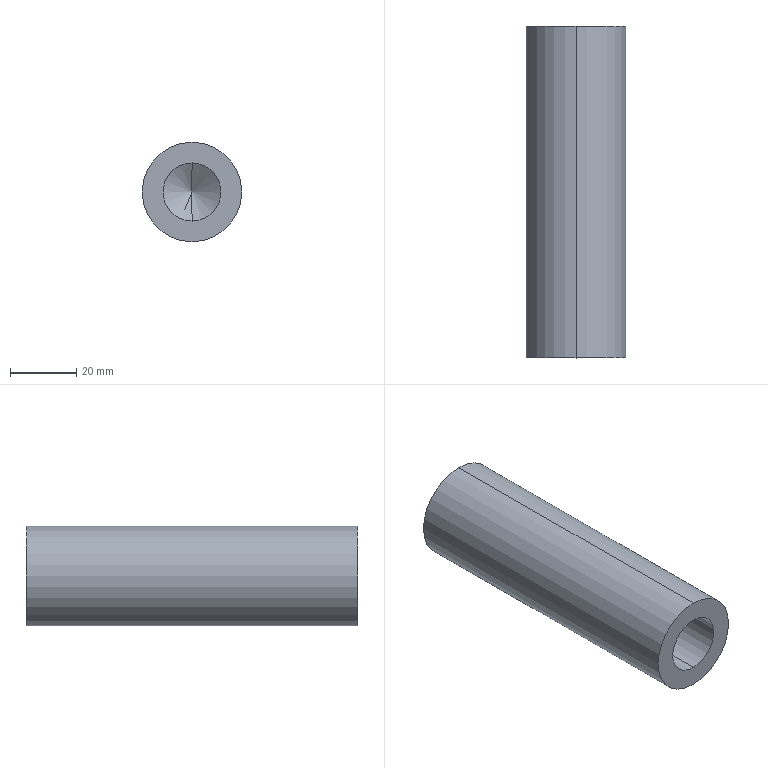Part | SolidWorks | features 3DProfileFeature 1, Extrusion 1, HoleWzd 1 | 1 solid | 8 faces | box 30 x 100 x 30 mm | volume 55231 mm3 | cylinder 4 | cone 2 | plane 2 | commonest cylinder face diameters 17.5 x2 30 x2
STEP:
#1=CARTESIAN_POINT('',(0.,12.5,8.75));
#2=VERTEX_POINT('',#1);
#3=CARTESIAN_POINT('',(0.,12.5,-8.75));
#4=VERTEX_POINT('',#3);
#5=CARTESIAN_POINT('',(0.,12.5,0.));
#6=DIRECTION('',(0.,-1.,0.));
#7=DIRECTION('',(0.,0.,-1.));
#8=AXIS2_PLACEMENT_3D('',#5,#6,#7);
#9=CIRCLE('',#8,8.75);
#10=EDGE_CURVE('',#2,#4,#9,.T.);
#11=ORIENTED_EDGE('',*,*,#10,.F.);
#12=CARTESIAN_POINT('',(0.,-50.,8.75));
#13=VERTEX_POINT('',#12);
#14=CARTESIAN_POINT('',(0.,-50.,8.75));
#15=DIRECTION('',(0.,-1.,0.));
#16=VECTOR('',#15,1000.);
#17=LINE('',#14,#16);
#18=EDGE_CURVE('',#2,#13,#17,.T.);
#19=ORIENTED_EDGE('',*,*,#18,.T.);
#20=CARTESIAN_POINT('',(0.,-50.,-8.75));
#21=VERTEX_POINT('',#20);
#22=CARTESIAN_POINT('',(0.,-50.,0.));
#23=DIRECTION('',(0.,-1.,0.));
#24=DIRECTION('',(0.,0.,-1.));
#25=AXIS2_PLACEMENT_3D('',#22,#23,#24);
#26=CIRCLE('',#25,8.75);
#27=EDGE_CURVE('',#13,#21,#26,.T.);
#28=ORIENTED_EDGE('',*,*,#27,.T.);
#29=CARTESIAN_POINT('',(0.,-50.,-8.75));
#30=DIRECTION('',(0.,-1.,0.));
#31=VECTOR('',#30,1000.);
#32=LINE('',#29,#31);
#33=EDGE_CURVE('',#4,#21,#32,.T.);
#34=ORIENTED_EDGE('',*,*,#33,.F.);
#35=EDGE_LOOP('',(#11,#19,#28,#34));
#36=FACE_OUTER_BOUND('',#35,.T.);
#37=CARTESIAN_POINT('',(0.,-50.,0.));
#38=DIRECTION('',(0.,-1.,0.));
#39=DIRECTION('',(0.,0.,-1.));
#40=AXIS2_PLACEMENT_3D('',#37,#38,#39);
#41=CYLINDRICAL_SURFACE('',#40,8.75);
#42=ADVANCED_FACE('',(#36),#41,.F.);
#43=CARTESIAN_POINT('',(0.,17.758,0.));
#44=VERTEX_POINT('',#43);
#45=CARTESIAN_POINT('',(0.,12.5,-8.75));
#46=DIRECTION('',(0.,-0.515,-0.8572));
#47=VECTOR('',#46,1000.);
#48=LINE('',#45,#47);
#49=EDGE_CURVE('',#44,#4,#48,.T.);
#50=ORIENTED_EDGE('',*,*,#49,.F.);
#51=CARTESIAN_POINT('',(0.,12.5,8.75));
#52=DIRECTION('',(0.,-0.515,0.8572));
#53=VECTOR('',#52,1000.);
#54=LINE('',#51,#53);
#55=EDGE_CURVE('',#44,#2,#54,.T.);
#56=ORIENTED_EDGE('',*,*,#55,.T.);
#57=ORIENTED_EDGE('',*,*,#10,.T.);
#58=EDGE_LOOP('',(#50,#56,#57));
#59=FACE_OUTER_BOUND('',#58,.T.);
#60=CARTESIAN_POINT('',(0.,12.5,0.));
#61=DIRECTION('',(0.,-1.,0.));
#62=DIRECTION('',(0.,0.,-1.));
#63=AXIS2_PLACEMENT_3D('',#60,#61,#62);
#64=CONICAL_SURFACE('',#63,8.75,1.03);
#65=ADVANCED_FACE('',(#59),#64,.F.);
#66=CARTESIAN_POINT('',(0.,50.,15.));
#67=VERTEX_POINT('',#66);
#68=CARTESIAN_POINT('',(0.,50.,-15.));
#69=VERTEX_POINT('',#68);
#70=CARTESIAN_POINT('',(0.,50.,0.));
#71=DIRECTION('',(0.,1.,0.));
#72=DIRECTION('',(0.,0.,1.));
#73=AXIS2_PLACEMENT_3D('',#70,#71,#72);
#74=CIRCLE('',#73,15.);
#75=EDGE_CURVE('',#67,#69,#74,.T.);
#76=ORIENTED_EDGE('',*,*,#75,.F.);
#77=CARTESIAN_POINT('',(0.,-50.,15.));
#78=VERTEX_POINT('',#77);
#79=CARTESIAN_POINT('',(0.,50.,15.));
#80=DIRECTION('',(0.,-1.,0.));
#81=VECTOR('',#80,1000.);
#82=LINE('',#79,#81);
#83=EDGE_CURVE('',#67,#78,#82,.T.);
#84=ORIENTED_EDGE('',*,*,#83,.T.);
#85=CARTESIAN_POINT('',(0.,-50.,-15.));
#86=VERTEX_POINT('',#85);
#87=CARTESIAN_POINT('',(0.,-50.,0.));
#88=DIRECTION('',(0.,1.,0.));
#89=DIRECTION('',(0.,0.,1.));
#90=AXIS2_PLACEMENT_3D('',#87,#88,#89);
#91=CIRCLE('',#90,15.);
#92=EDGE_CURVE('',#78,#86,#91,.T.);
#93=ORIENTED_EDGE('',*,*,#92,.T.);
#94=CARTESIAN_POINT('',(0.,50.,-15.));
#95=DIRECTION('',(0.,-1.,0.));
#96=VECTOR('',#95,1000.);
#97=LINE('',#94,#96);
#98=EDGE_CURVE('',#69,#86,#97,.T.);
#99=ORIENTED_EDGE('',*,*,#98,.F.);
#100=EDGE_LOOP('',(#76,#84,#93,#99));
#101=FACE_OUTER_BOUND('',#100,.T.);
#102=CARTESIAN_POINT('',(0.,50.,0.));
#103=DIRECTION('',(0.,-1.,0.));
#104=DIRECTION('',(0.,0.,-1.));
#105=AXIS2_PLACEMENT_3D('',#102,#103,#104);
#106=CYLINDRICAL_SURFACE('',#105,15.);
#107=ADVANCED_FACE('',(#101),#106,.T.);
#108=ORIENTED_EDGE('',*,*,#83,.F.);
#109=CARTESIAN_POINT('',(0.,50.,0.));
#110=DIRECTION('',(0.,1.,0.));
#111=DIRECTION('',(0.,0.,1.));
#112=AXIS2_PLACEMENT_3D('',#109,#110,#111);
#113=CIRCLE('',#112,15.);
#114=EDGE_CURVE('',#69,#67,#113,.T.);
#115=ORIENTED_EDGE('',*,*,#114,.F.);
#116=ORIENTED_EDGE('',*,*,#98,.T.);
#117=CARTESIAN_POINT('',(0.,-50.,0.));
#118=DIRECTION('',(0.,1.,0.));
#119=DIRECTION('',(0.,0.,1.));
#120=AXIS2_PLACEMENT_3D('',#117,#118,#119);
#121=CIRCLE('',#120,15.);
#122=EDGE_CURVE('',#86,#78,#121,.T.);
#123=ORIENTED_EDGE('',*,*,#122,.T.);
#124=EDGE_LOOP('',(#108,#115,#116,#123));
#125=FACE_OUTER_BOUND('',#124,.T.);
#126=CARTESIAN_POINT('',(0.,50.,0.));
#127=DIRECTION('',(0.,-1.,0.));
#128=DIRECTION('',(0.,0.,-1.));
#129=AXIS2_PLACEMENT_3D('',#126,#127,#128);
#130=CYLINDRICAL_SURFACE('',#129,15.);
#131=ADVANCED_FACE('',(#125),#130,.T.);
#132=ORIENTED_EDGE('',*,*,#114,.T.);
#133=ORIENTED_EDGE('',*,*,#75,.T.);
#134=EDGE_LOOP('',(#132,#133));
#135=FACE_OUTER_BOUND('',#134,.T.);
#136=CARTESIAN_POINT('',(0.,50.,0.));
#137=DIRECTION('',(0.,1.,0.));
#138=DIRECTION('',(0.,0.,1.));
#139=AXIS2_PLACEMENT_3D('',#136,#137,#138);
#140=PLANE('',#139);
#141=ADVANCED_FACE('',(#135),#140,.T.);
#142=CARTESIAN_POINT('',(0.,-50.,0.));
#143=DIRECTION('',(0.,-1.,0.));
#144=DIRECTION('',(0.,0.,-1.));
#145=AXIS2_PLACEMENT_3D('',#142,#143,#144);
#146=CIRCLE('',#145,8.75);
#147=EDGE_CURVE('',#21,#13,#146,.T.);
#148=ORIENTED_EDGE('',*,*,#147,.F.);
#149=ORIENTED_EDGE('',*,*,#27,.F.);
#150=EDGE_LOOP('',(#148,#149));
#151=FACE_BOUND('',#150,.T.);
#152=ORIENTED_EDGE('',*,*,#122,.F.);
#153=ORIENTED_EDGE('',*,*,#92,.F.);
#154=EDGE_LOOP('',(#152,#153));
#155=FACE_OUTER_BOUND('',#154,.T.);
#156=CARTESIAN_POINT('',(0.,-50.,0.));
#157=DIRECTION('',(0.,1.,0.));
#158=DIRECTION('',(0.,0.,1.));
#159=AXIS2_PLACEMENT_3D('',#156,#157,#158);
#160=PLANE('',#159);
#161=ADVANCED_FACE('',(#151,#155),#160,.F.);
#162=ORIENTED_EDGE('',*,*,#55,.F.);
#163=ORIENTED_EDGE('',*,*,#49,.T.);
#164=CARTESIAN_POINT('',(0.,12.5,0.));
#165=DIRECTION('',(0.,-1.,0.));
#166=DIRECTION('',(0.,0.,-1.));
#167=AXIS2_PLACEMENT_3D('',#164,#165,#166);
#168=CIRCLE('',#167,8.75);
#169=EDGE_CURVE('',#4,#2,#168,.T.);
#170=ORIENTED_EDGE('',*,*,#169,.T.);
#171=EDGE_LOOP('',(#162,#163,#170));
#172=FACE_OUTER_BOUND('',#171,.T.);
#173=CARTESIAN_POINT('',(0.,12.5,0.));
#174=DIRECTION('',(0.,-1.,0.));
#175=DIRECTION('',(0.,0.,-1.));
#176=AXIS2_PLACEMENT_3D('',#173,#174,#175);
#177=CONICAL_SURFACE('',#176,8.75,1.03);
#178=ADVANCED_FACE('',(#172),#177,.F.);
#179=ORIENTED_EDGE('',*,*,#18,.F.);
#180=ORIENTED_EDGE('',*,*,#169,.F.);
#181=ORIENTED_EDGE('',*,*,#33,.T.);
#182=ORIENTED_EDGE('',*,*,#147,.T.);
#183=EDGE_LOOP('',(#179,#180,#181,#182));
#184=FACE_OUTER_BOUND('',#183,.T.);
#185=CARTESIAN_POINT('',(0.,-50.,0.));
#186=DIRECTION('',(0.,-1.,0.));
#187=DIRECTION('',(0.,0.,-1.));
#188=AXIS2_PLACEMENT_3D('',#185,#186,#187);
#189=CYLINDRICAL_SURFACE('',#188,8.75);
#190=ADVANCED_FACE('',(#184),#189,.F.);
#191=CLOSED_SHELL('',(#42,#65,#107,#131,#141,#161,#178,#190));
#192=MANIFOLD_SOLID_BREP('',#191);
#193=CARTESIAN_POINT('',(0.,0.,0.));
#194=DIRECTION('',(0.,0.,1.));
#195=DIRECTION('',(1.,0.,0.));
#196=AXIS2_PLACEMENT_3D('',#193,#194,#195);
#197=(LENGTH_UNIT()NAMED_UNIT(*)SI_UNIT(.MILLI.,.METRE.));
#198=UNCERTAINTY_MEASURE_WITH_UNIT(LENGTH_MEASURE(0.00001),#197,'','');
#199=(NAMED_UNIT(*)PLANE_ANGLE_UNIT()SI_UNIT($,.RADIAN.));
#200=(NAMED_UNIT(*)SI_UNIT($,.STERADIAN.)SOLID_ANGLE_UNIT());
#201=(GEOMETRIC_REPRESENTATION_CONTEXT(3)GLOBAL_UNCERTAINTY_ASSIGNED_CONTEXT((#198))GLOBAL_UNIT_ASSIGNED_CONTEXT((#197,#199,#200))REPRESENTATION_CONTEXT('',''));
#202=ADVANCED_BREP_SHAPE_REPRESENTATION('',(#192,#196),#201);